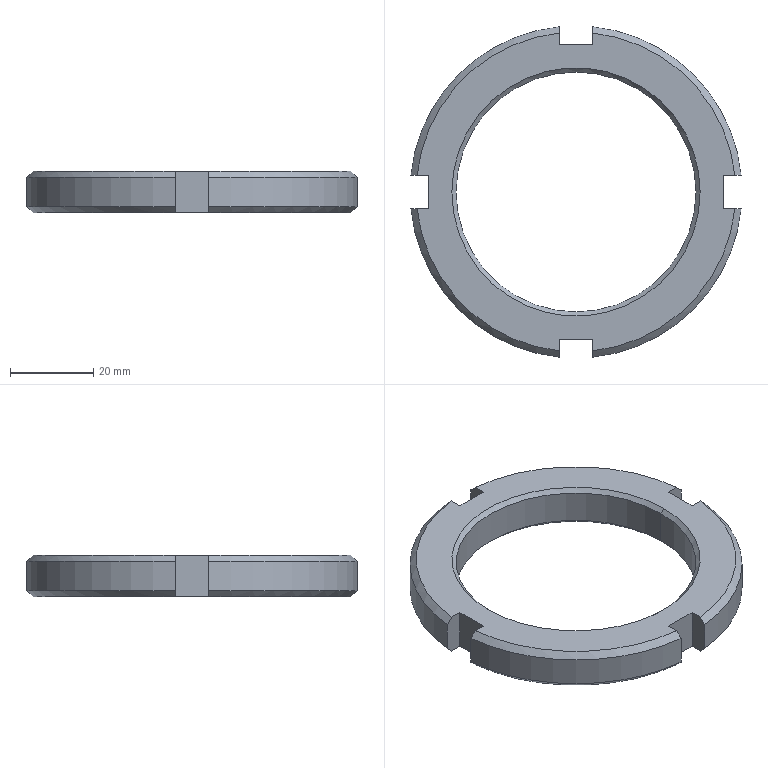Part | SolidWorks | features BaseBody 1 | 1 solid | 32 faces | box 79.599 x 79.599 x 10 mm | volume 21922 mm3 | plane 14 | cone 12 | cylinder 6 | commonest cylinder face diameters 80 x4 57.835 x2
STEP:
#1=CARTESIAN_POINT('',(-28.918,0.,9.));
#2=VERTEX_POINT('',#1);
#3=CARTESIAN_POINT('',(28.918,0.,9.));
#4=VERTEX_POINT('',#3);
#5=CARTESIAN_POINT('',(0.,0.,9.));
#6=DIRECTION('',(0.,0.,1.));
#7=DIRECTION('',(1.,0.,0.));
#8=AXIS2_PLACEMENT_3D('',#5,#6,#7);
#9=CIRCLE('',#8,28.918);
#10=EDGE_CURVE('',#2,#4,#9,.T.);
#11=ORIENTED_EDGE('',*,*,#10,.F.);
#12=CARTESIAN_POINT('',(-29.917,0.,10.));
#13=VERTEX_POINT('',#12);
#14=CARTESIAN_POINT('',(-28.918,0.,9.));
#15=DIRECTION('',(-0.7071,0.,0.7071));
#16=VECTOR('',#15,1000.);
#17=LINE('',#14,#16);
#18=EDGE_CURVE('',#2,#13,#17,.T.);
#19=ORIENTED_EDGE('',*,*,#18,.T.);
#20=CARTESIAN_POINT('',(29.917,0.,10.));
#21=VERTEX_POINT('',#20);
#22=CARTESIAN_POINT('',(0.,0.,10.));
#23=DIRECTION('',(0.,0.,-1.));
#24=DIRECTION('',(1.,0.,0.));
#25=AXIS2_PLACEMENT_3D('',#22,#23,#24);
#26=CIRCLE('',#25,29.918);
#27=EDGE_CURVE('',#21,#13,#26,.T.);
#28=ORIENTED_EDGE('',*,*,#27,.F.);
#29=CARTESIAN_POINT('',(28.918,0.,9.));
#30=DIRECTION('',(0.7071,0.,0.7071));
#31=VECTOR('',#30,1000.);
#32=LINE('',#29,#31);
#33=EDGE_CURVE('',#4,#21,#32,.T.);
#34=ORIENTED_EDGE('',*,*,#33,.F.);
#35=EDGE_LOOP('',(#11,#19,#28,#34));
#36=FACE_OUTER_BOUND('',#35,.T.);
#37=CARTESIAN_POINT('',(0.,0.,9.));
#38=DIRECTION('',(0.,0.,1.));
#39=DIRECTION('',(1.,0.,0.));
#40=AXIS2_PLACEMENT_3D('',#37,#38,#39);
#41=CONICAL_SURFACE('',#40,28.918,0.7854);
#42=ADVANCED_FACE('',(#36),#41,.F.);
#43=CARTESIAN_POINT('',(28.918,0.,1.));
#44=VERTEX_POINT('',#43);
#45=CARTESIAN_POINT('',(-28.918,0.,1.));
#46=VERTEX_POINT('',#45);
#47=CARTESIAN_POINT('',(0.,0.,1.));
#48=DIRECTION('',(0.,0.,-1.));
#49=DIRECTION('',(1.,0.,0.));
#50=AXIS2_PLACEMENT_3D('',#47,#48,#49);
#51=CIRCLE('',#50,28.918);
#52=EDGE_CURVE('',#44,#46,#51,.T.);
#53=ORIENTED_EDGE('',*,*,#52,.F.);
#54=CARTESIAN_POINT('',(29.918,0.,0.));
#55=VERTEX_POINT('',#54);
#56=CARTESIAN_POINT('',(29.918,0.,0.));
#57=DIRECTION('',(0.7071,0.,-0.7071));
#58=VECTOR('',#57,1000.);
#59=LINE('',#56,#58);
#60=EDGE_CURVE('',#44,#55,#59,.T.);
#61=ORIENTED_EDGE('',*,*,#60,.T.);
#62=CARTESIAN_POINT('',(-29.918,0.,0.));
#63=VERTEX_POINT('',#62);
#64=CARTESIAN_POINT('',(0.,0.,0.));
#65=DIRECTION('',(0.,0.,1.));
#66=DIRECTION('',(1.,0.,0.));
#67=AXIS2_PLACEMENT_3D('',#64,#65,#66);
#68=CIRCLE('',#67,29.918);
#69=EDGE_CURVE('',#63,#55,#68,.T.);
#70=ORIENTED_EDGE('',*,*,#69,.F.);
#71=CARTESIAN_POINT('',(-29.918,0.,0.));
#72=DIRECTION('',(-0.7071,0.,-0.7071));
#73=VECTOR('',#72,1000.);
#74=LINE('',#71,#73);
#75=EDGE_CURVE('',#46,#63,#74,.T.);
#76=ORIENTED_EDGE('',*,*,#75,.F.);
#77=EDGE_LOOP('',(#53,#61,#70,#76));
#78=FACE_OUTER_BOUND('',#77,.T.);
#79=CARTESIAN_POINT('',(0.,0.,0.));
#80=DIRECTION('',(0.,0.,-1.));
#81=DIRECTION('',(-1.,0.,0.));
#82=AXIS2_PLACEMENT_3D('',#79,#80,#81);
#83=CONICAL_SURFACE('',#82,29.918,0.7854);
#84=ADVANCED_FACE('',(#78),#83,.F.);
#85=ORIENTED_EDGE('',*,*,#10,.T.);
#86=CARTESIAN_POINT('',(28.918,0.,10.));
#87=DIRECTION('',(0.,0.,-1.));
#88=VECTOR('',#87,1000.);
#89=LINE('',#86,#88);
#90=EDGE_CURVE('',#4,#44,#89,.T.);
#91=ORIENTED_EDGE('',*,*,#90,.T.);
#92=ORIENTED_EDGE('',*,*,#52,.T.);
#93=CARTESIAN_POINT('',(-28.918,0.,10.));
#94=DIRECTION('',(0.,0.,-1.));
#95=VECTOR('',#94,1000.);
#96=LINE('',#93,#95);
#97=EDGE_CURVE('',#2,#46,#96,.T.);
#98=ORIENTED_EDGE('',*,*,#97,.F.);
#99=EDGE_LOOP('',(#85,#91,#92,#98));
#100=FACE_OUTER_BOUND('',#99,.T.);
#101=CARTESIAN_POINT('',(0.,0.,10.));
#102=DIRECTION('',(0.,0.,-1.));
#103=DIRECTION('',(-1.,0.,0.));
#104=AXIS2_PLACEMENT_3D('',#101,#102,#103);
#105=CYLINDRICAL_SURFACE('',#104,28.918);
#106=ADVANCED_FACE('',(#100),#105,.F.);
#107=CARTESIAN_POINT('',(4.,39.799,8.5));
#108=VERTEX_POINT('',#107);
#109=CARTESIAN_POINT('',(39.799,4.,8.5));
#110=VERTEX_POINT('',#109);
#111=CARTESIAN_POINT('',(0.,0.,8.5));
#112=DIRECTION('',(0.,0.,-1.));
#113=DIRECTION('',(1.,0.,0.));
#114=AXIS2_PLACEMENT_3D('',#111,#112,#113);
#115=CIRCLE('',#114,40.);
#116=EDGE_CURVE('',#108,#110,#115,.T.);
#117=ORIENTED_EDGE('',*,*,#116,.T.);
#118=CARTESIAN_POINT('',(39.799,4.,1.5));
#119=VERTEX_POINT('',#118);
#120=CARTESIAN_POINT('',(39.799,4.,0.));
#121=DIRECTION('',(0.,0.,1.));
#122=VECTOR('',#121,1000.);
#123=LINE('',#120,#122);
#124=EDGE_CURVE('',#119,#110,#123,.T.);
#125=ORIENTED_EDGE('',*,*,#124,.F.);
#126=CARTESIAN_POINT('',(4.,39.799,1.5));
#127=VERTEX_POINT('',#126);
#128=CARTESIAN_POINT('',(0.,0.,1.5));
#129=DIRECTION('',(0.,0.,1.));
#130=DIRECTION('',(1.,0.,0.));
#131=AXIS2_PLACEMENT_3D('',#128,#129,#130);
#132=CIRCLE('',#131,40.);
#133=EDGE_CURVE('',#119,#127,#132,.T.);
#134=ORIENTED_EDGE('',*,*,#133,.T.);
#135=CARTESIAN_POINT('',(4.,39.799,0.));
#136=DIRECTION('',(0.,0.,1.));
#137=VECTOR('',#136,1000.);
#138=LINE('',#135,#137);
#139=EDGE_CURVE('',#127,#108,#138,.T.);
#140=ORIENTED_EDGE('',*,*,#139,.T.);
#141=EDGE_LOOP('',(#117,#125,#134,#140));
#142=FACE_OUTER_BOUND('',#141,.T.);
#143=CARTESIAN_POINT('',(0.,0.,10.));
#144=DIRECTION('',(0.,0.,-1.));
#145=DIRECTION('',(-1.,0.,0.));
#146=AXIS2_PLACEMENT_3D('',#143,#144,#145);
#147=CYLINDRICAL_SURFACE('',#146,40.);
#148=ADVANCED_FACE('',(#142),#147,.T.);
#149=CARTESIAN_POINT('',(38.292,4.,10.));
#150=VERTEX_POINT('',#149);
#151=CARTESIAN_POINT('',(39.799,4.,8.5));
#152=CARTESIAN_POINT('',(39.408,4.,8.89));
#153=CARTESIAN_POINT('',(39.015,4.,9.28));
#154=CARTESIAN_POINT('',(38.623,4.,9.67));
#155=CARTESIAN_POINT('',(38.513,4.,9.78));
#156=CARTESIAN_POINT('',(38.402,4.,9.89));
#157=CARTESIAN_POINT('',(38.292,4.,10.));
#158=B_SPLINE_CURVE_WITH_KNOTS('',3,(#151,#152,#153,#154,#155,#156,#157),.UNSPECIFIED.,.F.,.F.,(4,3,4),(0.007217,0.008875,0.009343),.UNSPECIFIED.);
#159=EDGE_CURVE('',#110,#150,#158,.T.);
#160=ORIENTED_EDGE('',*,*,#159,.F.);
#161=ORIENTED_EDGE('',*,*,#116,.F.);
#162=CARTESIAN_POINT('',(4.,38.292,10.));
#163=VERTEX_POINT('',#162);
#164=CARTESIAN_POINT('',(4.,38.292,10.));
#165=CARTESIAN_POINT('',(4.,38.402,9.89));
#166=CARTESIAN_POINT('',(4.,38.513,9.78));
#167=CARTESIAN_POINT('',(4.,38.623,9.67));
#168=CARTESIAN_POINT('',(4.,39.015,9.28));
#169=CARTESIAN_POINT('',(4.,39.408,8.89));
#170=CARTESIAN_POINT('',(4.,39.799,8.5));
#171=B_SPLINE_CURVE_WITH_KNOTS('',3,(#164,#165,#166,#167,#168,#169,#170),.UNSPECIFIED.,.F.,.F.,(4,3,4),(0.008407,0.008875,0.01053),.UNSPECIFIED.);
#172=EDGE_CURVE('',#163,#108,#171,.T.);
#173=ORIENTED_EDGE('',*,*,#172,.F.);
#174=CARTESIAN_POINT('',(0.,0.,10.));
#175=DIRECTION('',(0.,0.,1.));
#176=DIRECTION('',(1.,0.,0.));
#177=AXIS2_PLACEMENT_3D('',#174,#175,#176);
#178=CIRCLE('',#177,38.5);
#179=EDGE_CURVE('',#150,#163,#178,.T.);
#180=ORIENTED_EDGE('',*,*,#179,.F.);
#181=EDGE_LOOP('',(#160,#161,#173,#180));
#182=FACE_OUTER_BOUND('',#181,.T.);
#183=CARTESIAN_POINT('',(0.,0.,10.));
#184=DIRECTION('',(0.,0.,-1.));
#185=DIRECTION('',(-1.,0.,0.));
#186=AXIS2_PLACEMENT_3D('',#183,#184,#185);
#187=CONICAL_SURFACE('',#186,38.5,0.7854);
#188=ADVANCED_FACE('',(#182),#187,.T.);
#189=CARTESIAN_POINT('',(38.292,4.,0.));
#190=VERTEX_POINT('',#189);
#191=CARTESIAN_POINT('',(38.292,4.,0.));
#192=CARTESIAN_POINT('',(38.402,4.,0.11));
#193=CARTESIAN_POINT('',(38.513,4.,0.22));
#194=CARTESIAN_POINT('',(38.623,4.,0.33));
#195=CARTESIAN_POINT('',(39.015,4.,0.72));
#196=CARTESIAN_POINT('',(39.408,4.,1.11));
#197=CARTESIAN_POINT('',(39.799,4.,1.5));
#198=B_SPLINE_CURVE_WITH_KNOTS('',3,(#191,#192,#193,#194,#195,#196,#197),.UNSPECIFIED.,.F.,.F.,(4,3,4),(0.008407,0.008875,0.01053),.UNSPECIFIED.);
#199=EDGE_CURVE('',#190,#119,#198,.T.);
#200=ORIENTED_EDGE('',*,*,#199,.F.);
#201=CARTESIAN_POINT('',(4.,38.292,0.));
#202=VERTEX_POINT('',#201);
#203=CARTESIAN_POINT('',(0.,0.,0.));
#204=DIRECTION('',(0.,0.,-1.));
#205=DIRECTION('',(1.,0.,0.));
#206=AXIS2_PLACEMENT_3D('',#203,#204,#205);
#207=CIRCLE('',#206,38.5);
#208=EDGE_CURVE('',#202,#190,#207,.T.);
#209=ORIENTED_EDGE('',*,*,#208,.F.);
#210=CARTESIAN_POINT('',(4.,39.799,1.5));
#211=CARTESIAN_POINT('',(4.,39.408,1.11));
#212=CARTESIAN_POINT('',(4.,39.015,0.72));
#213=CARTESIAN_POINT('',(4.,38.623,0.33));
#214=CARTESIAN_POINT('',(4.,38.513,0.22));
#215=CARTESIAN_POINT('',(4.,38.402,0.11));
#216=CARTESIAN_POINT('',(4.,38.292,0.));
#217=B_SPLINE_CURVE_WITH_KNOTS('',3,(#210,#211,#212,#213,#214,#215,#216),.UNSPECIFIED.,.F.,.F.,(4,3,4),(0.007217,0.008875,0.009343),.UNSPECIFIED.);
#218=EDGE_CURVE('',#127,#202,#217,.T.);
#219=ORIENTED_EDGE('',*,*,#218,.F.);
#220=ORIENTED_EDGE('',*,*,#133,.F.);
#221=EDGE_LOOP('',(#200,#209,#219,#220));
#222=FACE_OUTER_BOUND('',#221,.T.);
#223=CARTESIAN_POINT('',(0.,0.,1.5));
#224=DIRECTION('',(0.,0.,1.));
#225=DIRECTION('',(1.,0.,0.));
#226=AXIS2_PLACEMENT_3D('',#223,#224,#225);
#227=CONICAL_SURFACE('',#226,40.,0.7854);
#228=ADVANCED_FACE('',(#222),#227,.T.);
#229=CARTESIAN_POINT('',(-39.799,4.,8.5));
#230=VERTEX_POINT('',#229);
#231=CARTESIAN_POINT('',(-4.,39.799,8.5));
#232=VERTEX_POINT('',#231);
#233=CARTESIAN_POINT('',(0.,0.,8.5));
#234=DIRECTION('',(0.,0.,-1.));
#235=DIRECTION('',(1.,0.,0.));
#236=AXIS2_PLACEMENT_3D('',#233,#234,#235);
#237=CIRCLE('',#236,40.);
#238=EDGE_CURVE('',#230,#232,#237,.T.);
#239=ORIENTED_EDGE('',*,*,#238,.T.);
#240=CARTESIAN_POINT('',(-4.,39.799,1.5));
#241=VERTEX_POINT('',#240);
#242=CARTESIAN_POINT('',(-4.,39.799,0.));
#243=DIRECTION('',(0.,0.,1.));
#244=VECTOR('',#243,1000.);
#245=LINE('',#242,#244);
#246=EDGE_CURVE('',#241,#232,#245,.T.);
#247=ORIENTED_EDGE('',*,*,#246,.F.);
#248=CARTESIAN_POINT('',(-39.799,4.,1.5));
#249=VERTEX_POINT('',#248);
#250=CARTESIAN_POINT('',(0.,0.,1.5));
#251=DIRECTION('',(0.,0.,1.));
#252=DIRECTION('',(1.,0.,0.));
#253=AXIS2_PLACEMENT_3D('',#250,#251,#252);
#254=CIRCLE('',#253,40.);
#255=EDGE_CURVE('',#241,#249,#254,.T.);
#256=ORIENTED_EDGE('',*,*,#255,.T.);
#257=CARTESIAN_POINT('',(-39.799,4.,0.));
#258=DIRECTION('',(0.,0.,1.));
#259=VECTOR('',#258,1000.);
#260=LINE('',#257,#259);
#261=EDGE_CURVE('',#249,#230,#260,.T.);
#262=ORIENTED_EDGE('',*,*,#261,.T.);
#263=EDGE_LOOP('',(#239,#247,#256,#262));
#264=FACE_OUTER_BOUND('',#263,.T.);
#265=CARTESIAN_POINT('',(0.,0.,10.));
#266=DIRECTION('',(0.,0.,-1.));
#267=DIRECTION('',(-1.,0.,0.));
#268=AXIS2_PLACEMENT_3D('',#265,#266,#267);
#269=CYLINDRICAL_SURFACE('',#268,40.);
#270=ADVANCED_FACE('',(#264),#269,.T.);
#271=CARTESIAN_POINT('',(-4.,38.292,10.));
#272=VERTEX_POINT('',#271);
#273=CARTESIAN_POINT('',(-4.,39.799,8.5));
#274=CARTESIAN_POINT('',(-4.,39.408,8.89));
#275=CARTESIAN_POINT('',(-4.,39.015,9.28));
#276=CARTESIAN_POINT('',(-4.,38.623,9.67));
#277=CARTESIAN_POINT('',(-4.,38.513,9.78));
#278=CARTESIAN_POINT('',(-4.,38.402,9.89));
#279=CARTESIAN_POINT('',(-4.,38.292,10.));
#280=B_SPLINE_CURVE_WITH_KNOTS('',3,(#273,#274,#275,#276,#277,#278,#279),.UNSPECIFIED.,.F.,.F.,(4,3,4),(0.007217,0.008875,0.009343),.UNSPECIFIED.);
#281=EDGE_CURVE('',#232,#272,#280,.T.);
#282=ORIENTED_EDGE('',*,*,#281,.F.);
#283=ORIENTED_EDGE('',*,*,#238,.F.);
#284=CARTESIAN_POINT('',(-38.292,4.,10.));
#285=VERTEX_POINT('',#284);
#286=CARTESIAN_POINT('',(-38.292,4.,10.));
#287=CARTESIAN_POINT('',(-38.58,4.,9.713));
#288=CARTESIAN_POINT('',(-38.869,4.,9.426));
#289=CARTESIAN_POINT('',(-39.158,4.,9.139));
#290=CARTESIAN_POINT('',(-39.372,4.,8.926));
#291=CARTESIAN_POINT('',(-39.586,4.,8.713));
#292=CARTESIAN_POINT('',(-39.799,4.,8.5));
#293=B_SPLINE_CURVE_WITH_KNOTS('',3,(#286,#287,#288,#289,#290,#291,#292),.UNSPECIFIED.,.F.,.F.,(4,3,4),(0.007654,0.008875,0.009781),.UNSPECIFIED.);
#294=EDGE_CURVE('',#285,#230,#293,.T.);
#295=ORIENTED_EDGE('',*,*,#294,.F.);
#296=CARTESIAN_POINT('',(0.,0.,10.));
#297=DIRECTION('',(0.,0.,1.));
#298=DIRECTION('',(1.,0.,0.));
#299=AXIS2_PLACEMENT_3D('',#296,#297,#298);
#300=CIRCLE('',#299,38.5);
#301=EDGE_CURVE('',#272,#285,#300,.T.);
#302=ORIENTED_EDGE('',*,*,#301,.F.);
#303=EDGE_LOOP('',(#282,#283,#295,#302));
#304=FACE_OUTER_BOUND('',#303,.T.);
#305=CARTESIAN_POINT('',(0.,0.,10.));
#306=DIRECTION('',(0.,0.,-1.));
#307=DIRECTION('',(-1.,0.,0.));
#308=AXIS2_PLACEMENT_3D('',#305,#306,#307);
#309=CONICAL_SURFACE('',#308,38.5,0.7854);
#310=ADVANCED_FACE('',(#304),#309,.T.);
#311=CARTESIAN_POINT('',(-4.,38.292,0.));
#312=VERTEX_POINT('',#311);
#313=CARTESIAN_POINT('',(-4.,38.292,0.));
#314=CARTESIAN_POINT('',(-4.,38.402,0.11));
#315=CARTESIAN_POINT('',(-4.,38.513,0.22));
#316=CARTESIAN_POINT('',(-4.,38.623,0.33));
#317=CARTESIAN_POINT('',(-4.,39.015,0.72));
#318=CARTESIAN_POINT('',(-4.,39.408,1.11));
#319=CARTESIAN_POINT('',(-4.,39.799,1.5));
#320=B_SPLINE_CURVE_WITH_KNOTS('',3,(#313,#314,#315,#316,#317,#318,#319),.UNSPECIFIED.,.F.,.F.,(4,3,4),(0.008407,0.008875,0.01053),.UNSPECIFIED.);
#321=EDGE_CURVE('',#312,#241,#320,.T.);
#322=ORIENTED_EDGE('',*,*,#321,.F.);
#323=CARTESIAN_POINT('',(-38.292,4.,0.));
#324=VERTEX_POINT('',#323);
#325=CARTESIAN_POINT('',(0.,0.,0.));
#326=DIRECTION('',(0.,0.,-1.));
#327=DIRECTION('',(1.,0.,0.));
#328=AXIS2_PLACEMENT_3D('',#325,#326,#327);
#329=CIRCLE('',#328,38.5);
#330=EDGE_CURVE('',#324,#312,#329,.T.);
#331=ORIENTED_EDGE('',*,*,#330,.F.);
#332=CARTESIAN_POINT('',(-39.799,4.,1.5));
#333=CARTESIAN_POINT('',(-39.586,4.,1.287));
#334=CARTESIAN_POINT('',(-39.372,4.,1.074));
#335=CARTESIAN_POINT('',(-39.158,4.,0.8613));
#336=CARTESIAN_POINT('',(-38.869,4.,0.5742));
#337=CARTESIAN_POINT('',(-38.58,4.,0.2871));
#338=CARTESIAN_POINT('',(-38.292,4.,0.));
#339=B_SPLINE_CURVE_WITH_KNOTS('',3,(#332,#333,#334,#335,#336,#337,#338),.UNSPECIFIED.,.F.,.F.,(4,3,4),(0.00797,0.008875,0.0101),.UNSPECIFIED.);
#340=EDGE_CURVE('',#249,#324,#339,.T.);
#341=ORIENTED_EDGE('',*,*,#340,.F.);
#342=ORIENTED_EDGE('',*,*,#255,.F.);
#343=EDGE_LOOP('',(#322,#331,#341,#342));
#344=FACE_OUTER_BOUND('',#343,.T.);
#345=CARTESIAN_POINT('',(0.,0.,1.5));
#346=DIRECTION('',(0.,0.,1.));
#347=DIRECTION('',(1.,0.,0.));
#348=AXIS2_PLACEMENT_3D('',#345,#346,#347);
#349=CONICAL_SURFACE('',#348,40.,0.7854);
#350=ADVANCED_FACE('',(#344),#349,.T.);
#351=CARTESIAN_POINT('',(-4.,-39.799,8.5));
#352=VERTEX_POINT('',#351);
#353=CARTESIAN_POINT('',(-39.799,-4.,8.5));
#354=VERTEX_POINT('',#353);
#355=CARTESIAN_POINT('',(0.,0.,8.5));
#356=DIRECTION('',(0.,0.,-1.));
#357=DIRECTION('',(1.,0.,0.));
#358=AXIS2_PLACEMENT_3D('',#355,#356,#357);
#359=CIRCLE('',#358,40.);
#360=EDGE_CURVE('',#352,#354,#359,.T.);
#361=ORIENTED_EDGE('',*,*,#360,.T.);
#362=CARTESIAN_POINT('',(-39.799,-4.,1.5));
#363=VERTEX_POINT('',#362);
#364=CARTESIAN_POINT('',(-39.799,-4.,0.));
#365=DIRECTION('',(0.,0.,1.));
#366=VECTOR('',#365,1000.);
#367=LINE('',#364,#366);
#368=EDGE_CURVE('',#363,#354,#367,.T.);
#369=ORIENTED_EDGE('',*,*,#368,.F.);
#370=CARTESIAN_POINT('',(-4.,-39.799,1.5));
#371=VERTEX_POINT('',#370);
#372=CARTESIAN_POINT('',(0.,0.,1.5));
#373=DIRECTION('',(0.,0.,1.));
#374=DIRECTION('',(1.,0.,0.));
#375=AXIS2_PLACEMENT_3D('',#372,#373,#374);
#376=CIRCLE('',#375,40.);
#377=EDGE_CURVE('',#363,#371,#376,.T.);
#378=ORIENTED_EDGE('',*,*,#377,.T.);
#379=CARTESIAN_POINT('',(-4.,-39.799,0.));
#380=DIRECTION('',(0.,0.,1.));
#381=VECTOR('',#380,1000.);
#382=LINE('',#379,#381);
#383=EDGE_CURVE('',#371,#352,#382,.T.);
#384=ORIENTED_EDGE('',*,*,#383,.T.);
#385=EDGE_LOOP('',(#361,#369,#378,#384));
#386=FACE_OUTER_BOUND('',#385,.T.);
#387=CARTESIAN_POINT('',(0.,0.,10.));
#388=DIRECTION('',(0.,0.,-1.));
#389=DIRECTION('',(-1.,0.,0.));
#390=AXIS2_PLACEMENT_3D('',#387,#388,#389);
#391=CYLINDRICAL_SURFACE('',#390,40.);
#392=ADVANCED_FACE('',(#386),#391,.T.);
#393=CARTESIAN_POINT('',(-38.292,-4.,10.));
#394=VERTEX_POINT('',#393);
#395=CARTESIAN_POINT('',(-39.799,-4.,8.5));
#396=CARTESIAN_POINT('',(-39.586,-4.,8.713));
#397=CARTESIAN_POINT('',(-39.372,-4.,8.926));
#398=CARTESIAN_POINT('',(-39.158,-4.,9.139));
#399=CARTESIAN_POINT('',(-38.869,-4.,9.426));
#400=CARTESIAN_POINT('',(-38.58,-4.,9.713));
#401=CARTESIAN_POINT('',(-38.292,-4.,10.));
#402=B_SPLINE_CURVE_WITH_KNOTS('',3,(#395,#396,#397,#398,#399,#400,#401),.UNSPECIFIED.,.F.,.F.,(4,3,4),(0.00797,0.008875,0.0101),.UNSPECIFIED.);
#403=EDGE_CURVE('',#354,#394,#402,.T.);
#404=ORIENTED_EDGE('',*,*,#403,.F.);
#405=ORIENTED_EDGE('',*,*,#360,.F.);
#406=CARTESIAN_POINT('',(-4.,-38.292,10.));
#407=VERTEX_POINT('',#406);
#408=CARTESIAN_POINT('',(-4.,-38.292,10.));
#409=CARTESIAN_POINT('',(-4.,-38.794,9.5));
#410=CARTESIAN_POINT('',(-4.,-39.297,9.));
#411=CARTESIAN_POINT('',(-4.,-39.799,8.5));
#412=B_SPLINE_CURVE_WITH_KNOTS('',3,(#408,#409,#410,#411),.UNSPECIFIED.,.F.,.F.,(4,4),(0.,0.002127),.UNSPECIFIED.);
#413=EDGE_CURVE('',#407,#352,#412,.T.);
#414=ORIENTED_EDGE('',*,*,#413,.F.);
#415=CARTESIAN_POINT('',(0.,0.,10.));
#416=DIRECTION('',(0.,0.,1.));
#417=DIRECTION('',(1.,0.,0.));
#418=AXIS2_PLACEMENT_3D('',#415,#416,#417);
#419=CIRCLE('',#418,38.5);
#420=EDGE_CURVE('',#394,#407,#419,.T.);
#421=ORIENTED_EDGE('',*,*,#420,.F.);
#422=EDGE_LOOP('',(#404,#405,#414,#421));
#423=FACE_OUTER_BOUND('',#422,.T.);
#424=CARTESIAN_POINT('',(0.,0.,10.));
#425=DIRECTION('',(0.,0.,-1.));
#426=DIRECTION('',(-1.,0.,0.));
#427=AXIS2_PLACEMENT_3D('',#424,#425,#426);
#428=CONICAL_SURFACE('',#427,38.5,0.7854);
#429=ADVANCED_FACE('',(#423),#428,.T.);
#430=CARTESIAN_POINT('',(-38.292,-4.,0.));
#431=VERTEX_POINT('',#430);
#432=CARTESIAN_POINT('',(-38.292,-4.,0.));
#433=CARTESIAN_POINT('',(-38.58,-4.,0.2871));
#434=CARTESIAN_POINT('',(-38.869,-4.,0.5742));
#435=CARTESIAN_POINT('',(-39.158,-4.,0.8613));
#436=CARTESIAN_POINT('',(-39.372,-4.,1.074));
#437=CARTESIAN_POINT('',(-39.586,-4.,1.287));
#438=CARTESIAN_POINT('',(-39.799,-4.,1.5));
#439=B_SPLINE_CURVE_WITH_KNOTS('',3,(#432,#433,#434,#435,#436,#437,#438),.UNSPECIFIED.,.F.,.F.,(4,3,4),(0.007654,0.008875,0.009781),.UNSPECIFIED.);
#440=EDGE_CURVE('',#431,#363,#439,.T.);
#441=ORIENTED_EDGE('',*,*,#440,.F.);
#442=CARTESIAN_POINT('',(-4.,-38.292,0.));
#443=VERTEX_POINT('',#442);
#444=CARTESIAN_POINT('',(0.,0.,0.));
#445=DIRECTION('',(0.,0.,-1.));
#446=DIRECTION('',(1.,0.,0.));
#447=AXIS2_PLACEMENT_3D('',#444,#445,#446);
#448=CIRCLE('',#447,38.5);
#449=EDGE_CURVE('',#443,#431,#448,.T.);
#450=ORIENTED_EDGE('',*,*,#449,.F.);
#451=CARTESIAN_POINT('',(-4.,-39.799,1.5));
#452=CARTESIAN_POINT('',(-4.,-39.297,1.));
#453=CARTESIAN_POINT('',(-4.,-38.794,0.4999));
#454=CARTESIAN_POINT('',(-4.,-38.292,0.));
#455=B_SPLINE_CURVE_WITH_KNOTS('',3,(#451,#452,#453,#454),.UNSPECIFIED.,.F.,.F.,(4,4),(0.,0.002127),.UNSPECIFIED.);
#456=EDGE_CURVE('',#371,#443,#455,.T.);
#457=ORIENTED_EDGE('',*,*,#456,.F.);
#458=ORIENTED_EDGE('',*,*,#377,.F.);
#459=EDGE_LOOP('',(#441,#450,#457,#458));
#460=FACE_OUTER_BOUND('',#459,.T.);
#461=CARTESIAN_POINT('',(0.,0.,1.5));
#462=DIRECTION('',(0.,0.,1.));
#463=DIRECTION('',(1.,0.,0.));
#464=AXIS2_PLACEMENT_3D('',#461,#462,#463);
#465=CONICAL_SURFACE('',#464,40.,0.7854);
#466=ADVANCED_FACE('',(#460),#465,.T.);
#467=ORIENTED_EDGE('',*,*,#27,.T.);
#468=CARTESIAN_POINT('',(0.,0.,10.));
#469=DIRECTION('',(0.,0.,-1.));
#470=DIRECTION('',(1.,0.,0.));
#471=AXIS2_PLACEMENT_3D('',#468,#469,#470);
#472=CIRCLE('',#471,29.918);
#473=EDGE_CURVE('',#13,#21,#472,.T.);
#474=ORIENTED_EDGE('',*,*,#473,.T.);
#475=EDGE_LOOP('',(#467,#474));
#476=FACE_BOUND('',#475,.T.);
#477=CARTESIAN_POINT('',(35.549,4.,10.));
#478=VERTEX_POINT('',#477);
#479=CARTESIAN_POINT('',(35.549,4.,10.));
#480=DIRECTION('',(-1.,0.,0.));
#481=VECTOR('',#480,1000.);
#482=LINE('',#479,#481);
#483=EDGE_CURVE('',#150,#478,#482,.T.);
#484=ORIENTED_EDGE('',*,*,#483,.F.);
#485=ORIENTED_EDGE('',*,*,#179,.T.);
#486=CARTESIAN_POINT('',(4.,35.549,10.));
#487=VERTEX_POINT('',#486);
#488=CARTESIAN_POINT('',(4.,35.549,10.));
#489=DIRECTION('',(0.,1.,0.));
#490=VECTOR('',#489,1000.);
#491=LINE('',#488,#490);
#492=EDGE_CURVE('',#487,#163,#491,.T.);
#493=ORIENTED_EDGE('',*,*,#492,.F.);
#494=CARTESIAN_POINT('',(-4.,35.549,10.));
#495=VERTEX_POINT('',#494);
#496=CARTESIAN_POINT('',(4.,35.549,10.));
#497=DIRECTION('',(1.,0.,0.));
#498=VECTOR('',#497,1000.);
#499=LINE('',#496,#498);
#500=EDGE_CURVE('',#495,#487,#499,.T.);
#501=ORIENTED_EDGE('',*,*,#500,.F.);
#502=CARTESIAN_POINT('',(-4.,35.549,10.));
#503=DIRECTION('',(0.,-1.,0.));
#504=VECTOR('',#503,1000.);
#505=LINE('',#502,#504);
#506=EDGE_CURVE('',#272,#495,#505,.T.);
#507=ORIENTED_EDGE('',*,*,#506,.F.);
#508=ORIENTED_EDGE('',*,*,#301,.T.);
#509=CARTESIAN_POINT('',(-35.549,4.,10.));
#510=VERTEX_POINT('',#509);
#511=CARTESIAN_POINT('',(-35.549,4.,10.));
#512=DIRECTION('',(-1.,0.,0.));
#513=VECTOR('',#512,1000.);
#514=LINE('',#511,#513);
#515=EDGE_CURVE('',#510,#285,#514,.T.);
#516=ORIENTED_EDGE('',*,*,#515,.F.);
#517=CARTESIAN_POINT('',(-35.549,-4.,10.));
#518=VERTEX_POINT('',#517);
#519=CARTESIAN_POINT('',(-35.549,4.,10.));
#520=DIRECTION('',(0.,1.,0.));
#521=VECTOR('',#520,1000.);
#522=LINE('',#519,#521);
#523=EDGE_CURVE('',#518,#510,#522,.T.);
#524=ORIENTED_EDGE('',*,*,#523,.F.);
#525=CARTESIAN_POINT('',(-35.549,-4.,10.));
#526=DIRECTION('',(1.,0.,0.));
#527=VECTOR('',#526,1000.);
#528=LINE('',#525,#527);
#529=EDGE_CURVE('',#394,#518,#528,.T.);
#530=ORIENTED_EDGE('',*,*,#529,.F.);
#531=ORIENTED_EDGE('',*,*,#420,.T.);
#532=CARTESIAN_POINT('',(-4.,-35.549,10.));
#533=VERTEX_POINT('',#532);
#534=CARTESIAN_POINT('',(-4.,-35.549,10.));
#535=DIRECTION('',(0.,-1.,0.));
#536=VECTOR('',#535,1000.);
#537=LINE('',#534,#536);
#538=EDGE_CURVE('',#533,#407,#537,.T.);
#539=ORIENTED_EDGE('',*,*,#538,.F.);
#540=CARTESIAN_POINT('',(4.,-35.549,10.));
#541=VERTEX_POINT('',#540);
#542=CARTESIAN_POINT('',(-4.,-35.549,10.));
#543=DIRECTION('',(-1.,0.,0.));
#544=VECTOR('',#543,1000.);
#545=LINE('',#542,#544);
#546=EDGE_CURVE('',#541,#533,#545,.T.);
#547=ORIENTED_EDGE('',*,*,#546,.F.);
#548=CARTESIAN_POINT('',(4.,-38.292,10.));
#549=VERTEX_POINT('',#548);
#550=CARTESIAN_POINT('',(4.,-35.549,10.));
#551=DIRECTION('',(0.,1.,0.));
#552=VECTOR('',#551,1000.);
#553=LINE('',#550,#552);
#554=EDGE_CURVE('',#549,#541,#553,.T.);
#555=ORIENTED_EDGE('',*,*,#554,.F.);
#556=CARTESIAN_POINT('',(38.292,-4.,10.));
#557=VERTEX_POINT('',#556);
#558=CARTESIAN_POINT('',(0.,0.,10.));
#559=DIRECTION('',(0.,0.,1.));
#560=DIRECTION('',(1.,0.,0.));
#561=AXIS2_PLACEMENT_3D('',#558,#559,#560);
#562=CIRCLE('',#561,38.5);
#563=EDGE_CURVE('',#549,#557,#562,.T.);
#564=ORIENTED_EDGE('',*,*,#563,.T.);
#565=CARTESIAN_POINT('',(35.549,-4.,10.));
#566=VERTEX_POINT('',#565);
#567=CARTESIAN_POINT('',(35.549,-4.,10.));
#568=DIRECTION('',(1.,0.,0.));
#569=VECTOR('',#568,1000.);
#570=LINE('',#567,#569);
#571=EDGE_CURVE('',#566,#557,#570,.T.);
#572=ORIENTED_EDGE('',*,*,#571,.F.);
#573=CARTESIAN_POINT('',(35.549,-4.,10.));
#574=DIRECTION('',(0.,-1.,0.));
#575=VECTOR('',#574,1000.);
#576=LINE('',#573,#575);
#577=EDGE_CURVE('',#478,#566,#576,.T.);
#578=ORIENTED_EDGE('',*,*,#577,.F.);
#579=EDGE_LOOP('',(#484,#485,#493,#501,#507,#508,#516,#524,#530,#531,#539,#547,#555,#564,#572,#578));
#580=FACE_OUTER_BOUND('',#579,.T.);
#581=CARTESIAN_POINT('',(0.,0.,10.));
#582=DIRECTION('',(0.,0.,1.));
#583=DIRECTION('',(1.,0.,0.));
#584=AXIS2_PLACEMENT_3D('',#581,#582,#583);
#585=PLANE('',#584);
#586=ADVANCED_FACE('',(#476,#580),#585,.T.);
#587=ORIENTED_EDGE('',*,*,#69,.T.);
#588=CARTESIAN_POINT('',(0.,0.,0.));
#589=DIRECTION('',(0.,0.,1.));
#590=DIRECTION('',(1.,0.,0.));
#591=AXIS2_PLACEMENT_3D('',#588,#589,#590);
#592=CIRCLE('',#591,29.918);
#593=EDGE_CURVE('',#55,#63,#592,.T.);
#594=ORIENTED_EDGE('',*,*,#593,.T.);
#595=EDGE_LOOP('',(#587,#594));
#596=FACE_BOUND('',#595,.T.);
#597=ORIENTED_EDGE('',*,*,#208,.T.);
#598=CARTESIAN_POINT('',(35.549,4.,0.));
#599=VERTEX_POINT('',#598);
#600=CARTESIAN_POINT('',(35.549,4.,0.));
#601=DIRECTION('',(-1.,0.,0.));
#602=VECTOR('',#601,1000.);
#603=LINE('',#600,#602);
#604=EDGE_CURVE('',#190,#599,#603,.T.);
#605=ORIENTED_EDGE('',*,*,#604,.T.);
#606=CARTESIAN_POINT('',(35.549,-4.,0.));
#607=VERTEX_POINT('',#606);
#608=CARTESIAN_POINT('',(35.549,-4.,0.));
#609=DIRECTION('',(0.,-1.,0.));
#610=VECTOR('',#609,1000.);
#611=LINE('',#608,#610);
#612=EDGE_CURVE('',#599,#607,#611,.T.);
#613=ORIENTED_EDGE('',*,*,#612,.T.);
#614=CARTESIAN_POINT('',(38.292,-4.,0.));
#615=VERTEX_POINT('',#614);
#616=CARTESIAN_POINT('',(35.549,-4.,0.));
#617=DIRECTION('',(1.,0.,0.));
#618=VECTOR('',#617,1000.);
#619=LINE('',#616,#618);
#620=EDGE_CURVE('',#607,#615,#619,.T.);
#621=ORIENTED_EDGE('',*,*,#620,.T.);
#622=CARTESIAN_POINT('',(4.,-38.292,0.));
#623=VERTEX_POINT('',#622);
#624=CARTESIAN_POINT('',(0.,0.,0.));
#625=DIRECTION('',(0.,0.,-1.));
#626=DIRECTION('',(1.,0.,0.));
#627=AXIS2_PLACEMENT_3D('',#624,#625,#626);
#628=CIRCLE('',#627,38.5);
#629=EDGE_CURVE('',#615,#623,#628,.T.);
#630=ORIENTED_EDGE('',*,*,#629,.T.);
#631=CARTESIAN_POINT('',(4.,-35.549,0.));
#632=VERTEX_POINT('',#631);
#633=CARTESIAN_POINT('',(4.,-35.549,0.));
#634=DIRECTION('',(0.,1.,0.));
#635=VECTOR('',#634,1000.);
#636=LINE('',#633,#635);
#637=EDGE_CURVE('',#623,#632,#636,.T.);
#638=ORIENTED_EDGE('',*,*,#637,.T.);
#639=CARTESIAN_POINT('',(-4.,-35.549,0.));
#640=VERTEX_POINT('',#639);
#641=CARTESIAN_POINT('',(-4.,-35.549,0.));
#642=DIRECTION('',(-1.,0.,0.));
#643=VECTOR('',#642,1000.);
#644=LINE('',#641,#643);
#645=EDGE_CURVE('',#632,#640,#644,.T.);
#646=ORIENTED_EDGE('',*,*,#645,.T.);
#647=CARTESIAN_POINT('',(-4.,-35.549,0.));
#648=DIRECTION('',(0.,-1.,0.));
#649=VECTOR('',#648,1000.);
#650=LINE('',#647,#649);
#651=EDGE_CURVE('',#640,#443,#650,.T.);
#652=ORIENTED_EDGE('',*,*,#651,.T.);
#653=ORIENTED_EDGE('',*,*,#449,.T.);
#654=CARTESIAN_POINT('',(-35.549,-4.,0.));
#655=VERTEX_POINT('',#654);
#656=CARTESIAN_POINT('',(-35.549,-4.,0.));
#657=DIRECTION('',(1.,0.,0.));
#658=VECTOR('',#657,1000.);
#659=LINE('',#656,#658);
#660=EDGE_CURVE('',#431,#655,#659,.T.);
#661=ORIENTED_EDGE('',*,*,#660,.T.);
#662=CARTESIAN_POINT('',(-35.549,4.,0.));
#663=VERTEX_POINT('',#662);
#664=CARTESIAN_POINT('',(-35.549,4.,0.));
#665=DIRECTION('',(0.,1.,0.));
#666=VECTOR('',#665,1000.);
#667=LINE('',#664,#666);
#668=EDGE_CURVE('',#655,#663,#667,.T.);
#669=ORIENTED_EDGE('',*,*,#668,.T.);
#670=CARTESIAN_POINT('',(-35.549,4.,0.));
#671=DIRECTION('',(-1.,0.,0.));
#672=VECTOR('',#671,1000.);
#673=LINE('',#670,#672);
#674=EDGE_CURVE('',#663,#324,#673,.T.);
#675=ORIENTED_EDGE('',*,*,#674,.T.);
#676=ORIENTED_EDGE('',*,*,#330,.T.);
#677=CARTESIAN_POINT('',(-4.,35.549,0.));
#678=VERTEX_POINT('',#677);
#679=CARTESIAN_POINT('',(-4.,35.549,0.));
#680=DIRECTION('',(0.,-1.,0.));
#681=VECTOR('',#680,1000.);
#682=LINE('',#679,#681);
#683=EDGE_CURVE('',#312,#678,#682,.T.);
#684=ORIENTED_EDGE('',*,*,#683,.T.);
#685=CARTESIAN_POINT('',(4.,35.549,0.));
#686=VERTEX_POINT('',#685);
#687=CARTESIAN_POINT('',(4.,35.549,0.));
#688=DIRECTION('',(1.,0.,0.));
#689=VECTOR('',#688,1000.);
#690=LINE('',#687,#689);
#691=EDGE_CURVE('',#678,#686,#690,.T.);
#692=ORIENTED_EDGE('',*,*,#691,.T.);
#693=CARTESIAN_POINT('',(4.,35.549,0.));
#694=DIRECTION('',(0.,1.,0.));
#695=VECTOR('',#694,1000.);
#696=LINE('',#693,#695);
#697=EDGE_CURVE('',#686,#202,#696,.T.);
#698=ORIENTED_EDGE('',*,*,#697,.T.);
#699=EDGE_LOOP('',(#597,#605,#613,#621,#630,#638,#646,#652,#653,#661,#669,#675,#676,#684,#692,#698));
#700=FACE_OUTER_BOUND('',#699,.T.);
#701=CARTESIAN_POINT('',(0.,0.,0.));
#702=DIRECTION('',(0.,0.,1.));
#703=DIRECTION('',(1.,0.,0.));
#704=AXIS2_PLACEMENT_3D('',#701,#702,#703);
#705=PLANE('',#704);
#706=ADVANCED_FACE('',(#596,#700),#705,.F.);
#707=CARTESIAN_POINT('',(4.,-39.799,1.5));
#708=VERTEX_POINT('',#707);
#709=CARTESIAN_POINT('',(39.799,-4.,1.5));
#710=VERTEX_POINT('',#709);
#711=CARTESIAN_POINT('',(0.,0.,1.5));
#712=DIRECTION('',(0.,0.,1.));
#713=DIRECTION('',(1.,0.,0.));
#714=AXIS2_PLACEMENT_3D('',#711,#712,#713);
#715=CIRCLE('',#714,40.);
#716=EDGE_CURVE('',#708,#710,#715,.T.);
#717=ORIENTED_EDGE('',*,*,#716,.T.);
#718=CARTESIAN_POINT('',(39.799,-4.,8.5));
#719=VERTEX_POINT('',#718);
#720=CARTESIAN_POINT('',(39.799,-4.,0.));
#721=DIRECTION('',(0.,0.,1.));
#722=VECTOR('',#721,1000.);
#723=LINE('',#720,#722);
#724=EDGE_CURVE('',#710,#719,#723,.T.);
#725=ORIENTED_EDGE('',*,*,#724,.T.);
#726=CARTESIAN_POINT('',(4.,-39.799,8.5));
#727=VERTEX_POINT('',#726);
#728=CARTESIAN_POINT('',(0.,0.,8.5));
#729=DIRECTION('',(0.,0.,-1.));
#730=DIRECTION('',(1.,0.,0.));
#731=AXIS2_PLACEMENT_3D('',#728,#729,#730);
#732=CIRCLE('',#731,40.);
#733=EDGE_CURVE('',#719,#727,#732,.T.);
#734=ORIENTED_EDGE('',*,*,#733,.T.);
#735=CARTESIAN_POINT('',(4.,-39.799,0.));
#736=DIRECTION('',(0.,0.,1.));
#737=VECTOR('',#736,1000.);
#738=LINE('',#735,#737);
#739=EDGE_CURVE('',#708,#727,#738,.T.);
#740=ORIENTED_EDGE('',*,*,#739,.F.);
#741=EDGE_LOOP('',(#717,#725,#734,#740));
#742=FACE_OUTER_BOUND('',#741,.T.);
#743=CARTESIAN_POINT('',(0.,0.,10.));
#744=DIRECTION('',(0.,0.,-1.));
#745=DIRECTION('',(-1.,0.,0.));
#746=AXIS2_PLACEMENT_3D('',#743,#744,#745);
#747=CYLINDRICAL_SURFACE('',#746,40.);
#748=ADVANCED_FACE('',(#742),#747,.T.);
#749=ORIENTED_EDGE('',*,*,#90,.F.);
#750=CARTESIAN_POINT('',(0.,0.,9.));
#751=DIRECTION('',(0.,0.,1.));
#752=DIRECTION('',(1.,0.,0.));
#753=AXIS2_PLACEMENT_3D('',#750,#751,#752);
#754=CIRCLE('',#753,28.918);
#755=EDGE_CURVE('',#4,#2,#754,.T.);
#756=ORIENTED_EDGE('',*,*,#755,.T.);
#757=ORIENTED_EDGE('',*,*,#97,.T.);
#758=CARTESIAN_POINT('',(0.,0.,1.));
#759=DIRECTION('',(0.,0.,-1.));
#760=DIRECTION('',(1.,0.,0.));
#761=AXIS2_PLACEMENT_3D('',#758,#759,#760);
#762=CIRCLE('',#761,28.918);
#763=EDGE_CURVE('',#46,#44,#762,.T.);
#764=ORIENTED_EDGE('',*,*,#763,.T.);
#765=EDGE_LOOP('',(#749,#756,#757,#764));
#766=FACE_OUTER_BOUND('',#765,.T.);
#767=CARTESIAN_POINT('',(0.,0.,10.));
#768=DIRECTION('',(0.,0.,-1.));
#769=DIRECTION('',(-1.,0.,0.));
#770=AXIS2_PLACEMENT_3D('',#767,#768,#769);
#771=CYLINDRICAL_SURFACE('',#770,28.918);
#772=ADVANCED_FACE('',(#766),#771,.F.);
#773=ORIENTED_EDGE('',*,*,#546,.T.);
#774=CARTESIAN_POINT('',(-4.,-35.549,0.));
#775=DIRECTION('',(0.,0.,1.));
#776=VECTOR('',#775,1000.);
#777=LINE('',#774,#776);
#778=EDGE_CURVE('',#640,#533,#777,.T.);
#779=ORIENTED_EDGE('',*,*,#778,.F.);
#780=ORIENTED_EDGE('',*,*,#645,.F.);
#781=CARTESIAN_POINT('',(4.,-35.549,0.));
#782=DIRECTION('',(0.,0.,1.));
#783=VECTOR('',#782,1000.);
#784=LINE('',#781,#783);
#785=EDGE_CURVE('',#632,#541,#784,.T.);
#786=ORIENTED_EDGE('',*,*,#785,.T.);
#787=EDGE_LOOP('',(#773,#779,#780,#786));
#788=FACE_OUTER_BOUND('',#787,.T.);
#789=CARTESIAN_POINT('',(-4.,-35.549,0.));
#790=DIRECTION('',(0.,1.,0.));
#791=DIRECTION('',(0.,0.,1.));
#792=AXIS2_PLACEMENT_3D('',#789,#790,#791);
#793=PLANE('',#792);
#794=ADVANCED_FACE('',(#788),#793,.F.);
#795=ORIENTED_EDGE('',*,*,#739,.T.);
#796=CARTESIAN_POINT('',(4.,-39.799,8.5));
#797=CARTESIAN_POINT('',(4.,-39.297,9.));
#798=CARTESIAN_POINT('',(4.,-38.794,9.5));
#799=CARTESIAN_POINT('',(4.,-38.292,10.));
#800=B_SPLINE_CURVE_WITH_KNOTS('',3,(#796,#797,#798,#799),.UNSPECIFIED.,.F.,.F.,(4,4),(0.,0.002127),.UNSPECIFIED.);
#801=EDGE_CURVE('',#727,#549,#800,.T.);
#802=ORIENTED_EDGE('',*,*,#801,.T.);
#803=ORIENTED_EDGE('',*,*,#554,.T.);
#804=ORIENTED_EDGE('',*,*,#785,.F.);
#805=ORIENTED_EDGE('',*,*,#637,.F.);
#806=CARTESIAN_POINT('',(4.,-38.292,0.));
#807=CARTESIAN_POINT('',(4.,-38.794,0.4999));
#808=CARTESIAN_POINT('',(4.,-39.297,1.));
#809=CARTESIAN_POINT('',(4.,-39.799,1.5));
#810=B_SPLINE_CURVE_WITH_KNOTS('',3,(#806,#807,#808,#809),.UNSPECIFIED.,.F.,.F.,(4,4),(0.,0.002127),.UNSPECIFIED.);
#811=EDGE_CURVE('',#623,#708,#810,.T.);
#812=ORIENTED_EDGE('',*,*,#811,.T.);
#813=EDGE_LOOP('',(#795,#802,#803,#804,#805,#812));
#814=FACE_OUTER_BOUND('',#813,.T.);
#815=CARTESIAN_POINT('',(4.,-35.549,0.));
#816=DIRECTION('',(1.,0.,0.));
#817=DIRECTION('',(0.,1.,0.));
#818=AXIS2_PLACEMENT_3D('',#815,#816,#817);
#819=PLANE('',#818);
#820=ADVANCED_FACE('',(#814),#819,.F.);
#821=ORIENTED_EDGE('',*,*,#538,.T.);
#822=ORIENTED_EDGE('',*,*,#413,.T.);
#823=ORIENTED_EDGE('',*,*,#383,.F.);
#824=ORIENTED_EDGE('',*,*,#456,.T.);
#825=ORIENTED_EDGE('',*,*,#651,.F.);
#826=ORIENTED_EDGE('',*,*,#778,.T.);
#827=EDGE_LOOP('',(#821,#822,#823,#824,#825,#826));
#828=FACE_OUTER_BOUND('',#827,.T.);
#829=CARTESIAN_POINT('',(-4.,-35.549,0.));
#830=DIRECTION('',(-1.,0.,0.));
#831=DIRECTION('',(0.,-1.,0.));
#832=AXIS2_PLACEMENT_3D('',#829,#830,#831);
#833=PLANE('',#832);
#834=ADVANCED_FACE('',(#828),#833,.F.);
#835=CARTESIAN_POINT('',(38.292,-4.,10.));
#836=CARTESIAN_POINT('',(38.402,-4.,9.89));
#837=CARTESIAN_POINT('',(38.513,-4.,9.78));
#838=CARTESIAN_POINT('',(38.623,-4.,9.67));
#839=CARTESIAN_POINT('',(39.015,-4.,9.28));
#840=CARTESIAN_POINT('',(39.408,-4.,8.89));
#841=CARTESIAN_POINT('',(39.799,-4.,8.5));
#842=B_SPLINE_CURVE_WITH_KNOTS('',3,(#835,#836,#837,#838,#839,#840,#841),.UNSPECIFIED.,.F.,.F.,(4,3,4),(0.008407,0.008875,0.01053),.UNSPECIFIED.);
#843=EDGE_CURVE('',#557,#719,#842,.T.);
#844=ORIENTED_EDGE('',*,*,#843,.F.);
#845=ORIENTED_EDGE('',*,*,#563,.F.);
#846=ORIENTED_EDGE('',*,*,#801,.F.);
#847=ORIENTED_EDGE('',*,*,#733,.F.);
#848=EDGE_LOOP('',(#844,#845,#846,#847));
#849=FACE_OUTER_BOUND('',#848,.T.);
#850=CARTESIAN_POINT('',(0.,0.,10.));
#851=DIRECTION('',(0.,0.,-1.));
#852=DIRECTION('',(-1.,0.,0.));
#853=AXIS2_PLACEMENT_3D('',#850,#851,#852);
#854=CONICAL_SURFACE('',#853,38.5,0.7854);
#855=ADVANCED_FACE('',(#849),#854,.T.);
#856=CARTESIAN_POINT('',(39.799,-4.,1.5));
#857=CARTESIAN_POINT('',(39.408,-4.,1.11));
#858=CARTESIAN_POINT('',(39.015,-4.,0.72));
#859=CARTESIAN_POINT('',(38.623,-4.,0.33));
#860=CARTESIAN_POINT('',(38.513,-4.,0.22));
#861=CARTESIAN_POINT('',(38.402,-4.,0.11));
#862=CARTESIAN_POINT('',(38.292,-4.,0.));
#863=B_SPLINE_CURVE_WITH_KNOTS('',3,(#856,#857,#858,#859,#860,#861,#862),.UNSPECIFIED.,.F.,.F.,(4,3,4),(0.007217,0.008875,0.009343),.UNSPECIFIED.);
#864=EDGE_CURVE('',#710,#615,#863,.T.);
#865=ORIENTED_EDGE('',*,*,#864,.F.);
#866=ORIENTED_EDGE('',*,*,#716,.F.);
#867=ORIENTED_EDGE('',*,*,#811,.F.);
#868=ORIENTED_EDGE('',*,*,#629,.F.);
#869=EDGE_LOOP('',(#865,#866,#867,#868));
#870=FACE_OUTER_BOUND('',#869,.T.);
#871=CARTESIAN_POINT('',(0.,0.,1.5));
#872=DIRECTION('',(0.,0.,1.));
#873=DIRECTION('',(1.,0.,0.));
#874=AXIS2_PLACEMENT_3D('',#871,#872,#873);
#875=CONICAL_SURFACE('',#874,40.,0.7854);
#876=ADVANCED_FACE('',(#870),#875,.T.);
#877=ORIENTED_EDGE('',*,*,#523,.T.);
#878=CARTESIAN_POINT('',(-35.549,4.,0.));
#879=DIRECTION('',(0.,0.,1.));
#880=VECTOR('',#879,1000.);
#881=LINE('',#878,#880);
#882=EDGE_CURVE('',#663,#510,#881,.T.);
#883=ORIENTED_EDGE('',*,*,#882,.F.);
#884=ORIENTED_EDGE('',*,*,#668,.F.);
#885=CARTESIAN_POINT('',(-35.549,-4.,0.));
#886=DIRECTION('',(0.,0.,1.));
#887=VECTOR('',#886,1000.);
#888=LINE('',#885,#887);
#889=EDGE_CURVE('',#655,#518,#888,.T.);
#890=ORIENTED_EDGE('',*,*,#889,.T.);
#891=EDGE_LOOP('',(#877,#883,#884,#890));
#892=FACE_OUTER_BOUND('',#891,.T.);
#893=CARTESIAN_POINT('',(-35.549,4.,0.));
#894=DIRECTION('',(1.,0.,0.));
#895=DIRECTION('',(0.,1.,0.));
#896=AXIS2_PLACEMENT_3D('',#893,#894,#895);
#897=PLANE('',#896);
#898=ADVANCED_FACE('',(#892),#897,.F.);
#899=ORIENTED_EDGE('',*,*,#403,.T.);
#900=ORIENTED_EDGE('',*,*,#529,.T.);
#901=ORIENTED_EDGE('',*,*,#889,.F.);
#902=ORIENTED_EDGE('',*,*,#660,.F.);
#903=ORIENTED_EDGE('',*,*,#440,.T.);
#904=ORIENTED_EDGE('',*,*,#368,.T.);
#905=EDGE_LOOP('',(#899,#900,#901,#902,#903,#904));
#906=FACE_OUTER_BOUND('',#905,.T.);
#907=CARTESIAN_POINT('',(-35.549,-4.,0.));
#908=DIRECTION('',(0.,-1.,0.));
#909=DIRECTION('',(1.,0.,0.));
#910=AXIS2_PLACEMENT_3D('',#907,#908,#909);
#911=PLANE('',#910);
#912=ADVANCED_FACE('',(#906),#911,.F.);
#913=ORIENTED_EDGE('',*,*,#294,.T.);
#914=ORIENTED_EDGE('',*,*,#261,.F.);
#915=ORIENTED_EDGE('',*,*,#340,.T.);
#916=ORIENTED_EDGE('',*,*,#674,.F.);
#917=ORIENTED_EDGE('',*,*,#882,.T.);
#918=ORIENTED_EDGE('',*,*,#515,.T.);
#919=EDGE_LOOP('',(#913,#914,#915,#916,#917,#918));
#920=FACE_OUTER_BOUND('',#919,.T.);
#921=CARTESIAN_POINT('',(-35.549,4.,0.));
#922=DIRECTION('',(0.,1.,0.));
#923=DIRECTION('',(-1.,0.,0.));
#924=AXIS2_PLACEMENT_3D('',#921,#922,#923);
#925=PLANE('',#924);
#926=ADVANCED_FACE('',(#920),#925,.F.);
#927=ORIENTED_EDGE('',*,*,#500,.T.);
#928=CARTESIAN_POINT('',(4.,35.549,0.));
#929=DIRECTION('',(0.,0.,1.));
#930=VECTOR('',#929,1000.);
#931=LINE('',#928,#930);
#932=EDGE_CURVE('',#686,#487,#931,.T.);
#933=ORIENTED_EDGE('',*,*,#932,.F.);
#934=ORIENTED_EDGE('',*,*,#691,.F.);
#935=CARTESIAN_POINT('',(-4.,35.549,0.));
#936=DIRECTION('',(0.,0.,1.));
#937=VECTOR('',#936,1000.);
#938=LINE('',#935,#937);
#939=EDGE_CURVE('',#678,#495,#938,.T.);
#940=ORIENTED_EDGE('',*,*,#939,.T.);
#941=EDGE_LOOP('',(#927,#933,#934,#940));
#942=FACE_OUTER_BOUND('',#941,.T.);
#943=CARTESIAN_POINT('',(4.,35.549,0.));
#944=DIRECTION('',(0.,-1.,0.));
#945=DIRECTION('',(1.,0.,0.));
#946=AXIS2_PLACEMENT_3D('',#943,#944,#945);
#947=PLANE('',#946);
#948=ADVANCED_FACE('',(#942),#947,.F.);
#949=ORIENTED_EDGE('',*,*,#281,.T.);
#950=ORIENTED_EDGE('',*,*,#506,.T.);
#951=ORIENTED_EDGE('',*,*,#939,.F.);
#952=ORIENTED_EDGE('',*,*,#683,.F.);
#953=ORIENTED_EDGE('',*,*,#321,.T.);
#954=ORIENTED_EDGE('',*,*,#246,.T.);
#955=EDGE_LOOP('',(#949,#950,#951,#952,#953,#954));
#956=FACE_OUTER_BOUND('',#955,.T.);
#957=CARTESIAN_POINT('',(-4.,35.549,0.));
#958=DIRECTION('',(-1.,0.,0.));
#959=DIRECTION('',(0.,-1.,0.));
#960=AXIS2_PLACEMENT_3D('',#957,#958,#959);
#961=PLANE('',#960);
#962=ADVANCED_FACE('',(#956),#961,.F.);
#963=ORIENTED_EDGE('',*,*,#172,.T.);
#964=ORIENTED_EDGE('',*,*,#139,.F.);
#965=ORIENTED_EDGE('',*,*,#218,.T.);
#966=ORIENTED_EDGE('',*,*,#697,.F.);
#967=ORIENTED_EDGE('',*,*,#932,.T.);
#968=ORIENTED_EDGE('',*,*,#492,.T.);
#969=EDGE_LOOP('',(#963,#964,#965,#966,#967,#968));
#970=FACE_OUTER_BOUND('',#969,.T.);
#971=CARTESIAN_POINT('',(4.,35.549,0.));
#972=DIRECTION('',(1.,0.,0.));
#973=DIRECTION('',(0.,1.,0.));
#974=AXIS2_PLACEMENT_3D('',#971,#972,#973);
#975=PLANE('',#974);
#976=ADVANCED_FACE('',(#970),#975,.F.);
#977=ORIENTED_EDGE('',*,*,#577,.T.);
#978=CARTESIAN_POINT('',(35.549,-4.,0.));
#979=DIRECTION('',(0.,0.,1.));
#980=VECTOR('',#979,1000.);
#981=LINE('',#978,#980);
#982=EDGE_CURVE('',#607,#566,#981,.T.);
#983=ORIENTED_EDGE('',*,*,#982,.F.);
#984=ORIENTED_EDGE('',*,*,#612,.F.);
#985=CARTESIAN_POINT('',(35.549,4.,0.));
#986=DIRECTION('',(0.,0.,1.));
#987=VECTOR('',#986,1000.);
#988=LINE('',#985,#987);
#989=EDGE_CURVE('',#599,#478,#988,.T.);
#990=ORIENTED_EDGE('',*,*,#989,.T.);
#991=EDGE_LOOP('',(#977,#983,#984,#990));
#992=FACE_OUTER_BOUND('',#991,.T.);
#993=CARTESIAN_POINT('',(35.549,-4.,0.));
#994=DIRECTION('',(-1.,0.,0.));
#995=DIRECTION('',(0.,-1.,0.));
#996=AXIS2_PLACEMENT_3D('',#993,#994,#995);
#997=PLANE('',#996);
#998=ADVANCED_FACE('',(#992),#997,.F.);
#999=ORIENTED_EDGE('',*,*,#159,.T.);
#1000=ORIENTED_EDGE('',*,*,#483,.T.);
#1001=ORIENTED_EDGE('',*,*,#989,.F.);
#1002=ORIENTED_EDGE('',*,*,#604,.F.);
#1003=ORIENTED_EDGE('',*,*,#199,.T.);
#1004=ORIENTED_EDGE('',*,*,#124,.T.);
#1005=EDGE_LOOP('',(#999,#1000,#1001,#1002,#1003,#1004));
#1006=FACE_OUTER_BOUND('',#1005,.T.);
#1007=CARTESIAN_POINT('',(35.549,4.,0.));
#1008=DIRECTION('',(0.,1.,0.));
#1009=DIRECTION('',(-1.,0.,0.));
#1010=AXIS2_PLACEMENT_3D('',#1007,#1008,#1009);
#1011=PLANE('',#1010);
#1012=ADVANCED_FACE('',(#1006),#1011,.F.);
#1013=ORIENTED_EDGE('',*,*,#843,.T.);
#1014=ORIENTED_EDGE('',*,*,#724,.F.);
#1015=ORIENTED_EDGE('',*,*,#864,.T.);
#1016=ORIENTED_EDGE('',*,*,#620,.F.);
#1017=ORIENTED_EDGE('',*,*,#982,.T.);
#1018=ORIENTED_EDGE('',*,*,#571,.T.);
#1019=EDGE_LOOP('',(#1013,#1014,#1015,#1016,#1017,#1018));
#1020=FACE_OUTER_BOUND('',#1019,.T.);
#1021=CARTESIAN_POINT('',(35.549,-4.,0.));
#1022=DIRECTION('',(0.,-1.,0.));
#1023=DIRECTION('',(1.,0.,0.));
#1024=AXIS2_PLACEMENT_3D('',#1021,#1022,#1023);
#1025=PLANE('',#1024);
#1026=ADVANCED_FACE('',(#1020),#1025,.F.);
#1027=ORIENTED_EDGE('',*,*,#60,.F.);
#1028=ORIENTED_EDGE('',*,*,#763,.F.);
#1029=ORIENTED_EDGE('',*,*,#75,.T.);
#1030=ORIENTED_EDGE('',*,*,#593,.F.);
#1031=EDGE_LOOP('',(#1027,#1028,#1029,#1030));
#1032=FACE_OUTER_BOUND('',#1031,.T.);
#1033=CARTESIAN_POINT('',(0.,0.,0.));
#1034=DIRECTION('',(0.,0.,-1.));
#1035=DIRECTION('',(-1.,0.,0.));
#1036=AXIS2_PLACEMENT_3D('',#1033,#1034,#1035);
#1037=CONICAL_SURFACE('',#1036,29.918,0.7854);
#1038=ADVANCED_FACE('',(#1032),#1037,.F.);
#1039=ORIENTED_EDGE('',*,*,#18,.F.);
#1040=ORIENTED_EDGE('',*,*,#755,.F.);
#1041=ORIENTED_EDGE('',*,*,#33,.T.);
#1042=ORIENTED_EDGE('',*,*,#473,.F.);
#1043=EDGE_LOOP('',(#1039,#1040,#1041,#1042));
#1044=FACE_OUTER_BOUND('',#1043,.T.);
#1045=CARTESIAN_POINT('',(0.,0.,9.));
#1046=DIRECTION('',(0.,0.,1.));
#1047=DIRECTION('',(1.,0.,0.));
#1048=AXIS2_PLACEMENT_3D('',#1045,#1046,#1047);
#1049=CONICAL_SURFACE('',#1048,28.918,0.7854);
#1050=ADVANCED_FACE('',(#1044),#1049,.F.);
#1051=CLOSED_SHELL('',(#42,#84,#106,#148,#188,#228,#270,#310,#350,#392,#429,#466,#586,#706,#748,#772,#794,#820,#834,#855,#876,#898,#912,#926,#948,#962,#976,#998,#1012,#1026,#1038,#1050));
#1052=MANIFOLD_SOLID_BREP('',#1051);
#1053=CARTESIAN_POINT('',(0.,0.,0.));
#1054=DIRECTION('',(0.,0.,1.));
#1055=DIRECTION('',(1.,0.,0.));
#1056=AXIS2_PLACEMENT_3D('',#1053,#1054,#1055);
#1057=(LENGTH_UNIT()NAMED_UNIT(*)SI_UNIT(.MILLI.,.METRE.));
#1058=UNCERTAINTY_MEASURE_WITH_UNIT(LENGTH_MEASURE(0.00001),#1057,'','');
#1059=(NAMED_UNIT(*)PLANE_ANGLE_UNIT()SI_UNIT($,.RADIAN.));
#1060=(NAMED_UNIT(*)SI_UNIT($,.STERADIAN.)SOLID_ANGLE_UNIT());
#1061=(GEOMETRIC_REPRESENTATION_CONTEXT(3)GLOBAL_UNCERTAINTY_ASSIGNED_CONTEXT((#1058))GLOBAL_UNIT_ASSIGNED_CONTEXT((#1057,#1059,#1060))REPRESENTATION_CONTEXT('',''));
#1062=ADVANCED_BREP_SHAPE_REPRESENTATION('',(#1052,#1056),#1061);